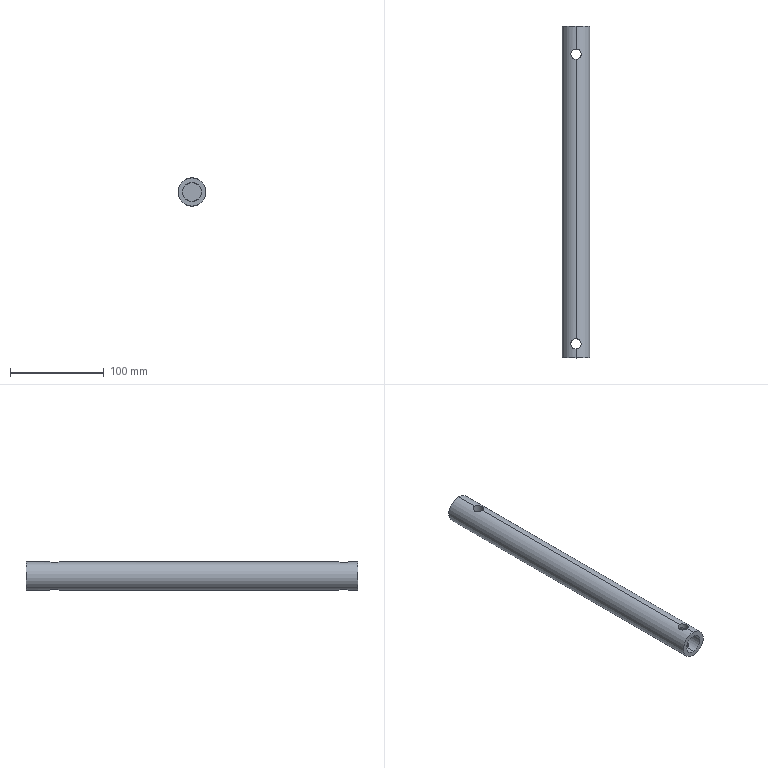Part | SolidWorks | features ICE 2, Extrusion 1, MoveFace 1 | 1 solid | 13 faces | box 30 x 354 x 30 mm | volume 230741 mm3 | cylinder 10 | plane 3 | commonest cylinder face diameters 11 x6 20 x2 30 x2
STEP:
#1=CARTESIAN_POINT('',(-5.5,324.,-13.955));
#2=VERTEX_POINT('',#1);
#3=CARTESIAN_POINT('',(0.,318.5,-15.));
#4=VERTEX_POINT('',#3);
#5=CARTESIAN_POINT('',(-5.5,324.,-13.955));
#6=CARTESIAN_POINT('',(-5.5,323.818,-13.955));
#7=CARTESIAN_POINT('',(-5.491,323.634,-13.959));
#8=CARTESIAN_POINT('',(-5.455,323.272,-13.973));
#9=CARTESIAN_POINT('',(-5.428,323.093,-13.984));
#10=CARTESIAN_POINT('',(-5.321,322.562,-14.025));
#11=CARTESIAN_POINT('',(-5.215,322.214,-14.065));
#12=CARTESIAN_POINT('',(-4.936,321.547,-14.165));
#13=CARTESIAN_POINT('',(-4.766,321.232,-14.224));
#14=CARTESIAN_POINT('',(-4.368,320.639,-14.352));
#15=CARTESIAN_POINT('',(-4.137,320.358,-14.421));
#16=CARTESIAN_POINT('',(-3.633,319.855,-14.556));
#17=CARTESIAN_POINT('',(-3.358,319.63,-14.622));
#18=CARTESIAN_POINT('',(-2.91,319.33,-14.716));
#19=CARTESIAN_POINT('',(-2.755,319.236,-14.746));
#20=CARTESIAN_POINT('',(-2.438,319.067,-14.801));
#21=CARTESIAN_POINT('',(-2.277,318.99,-14.827));
#22=CARTESIAN_POINT('',(-1.782,318.785,-14.897));
#23=CARTESIAN_POINT('',(-1.44,318.679,-14.935));
#24=CARTESIAN_POINT('',(-0.904,318.572,-14.974));
#25=CARTESIAN_POINT('',(-0.7225,318.545,-14.984));
#26=CARTESIAN_POINT('',(-0.3614,318.509,-14.997));
#27=CARTESIAN_POINT('',(-0.1808,318.5,-15.));
#28=CARTESIAN_POINT('',(0.,318.5,-15.));
#29=B_SPLINE_CURVE_WITH_KNOTS('',3,(#5,#6,#7,#8,#9,#10,#11,#12,#13,#14,#15,#16,#17,#18,#19,#20,#21,#22,#23,#24,#25,#26,#27,#28),.UNSPECIFIED.,.F.,.F.,(4,2,2,2,2,2,2,2,2,2,2,4),(0.02696,0.02751,0.02805,0.02913,0.03022,0.0313,0.03239,0.03293,0.03347,0.03456,0.0351,0.03564),.UNSPECIFIED.);
#30=EDGE_CURVE('',#2,#4,#29,.T.);
#31=ORIENTED_EDGE('',*,*,#30,.F.);
#32=CARTESIAN_POINT('',(-5.5,324.,13.955));
#33=VERTEX_POINT('',#32);
#34=CARTESIAN_POINT('',(-5.5,324.,-126.));
#35=DIRECTION('',(0.,0.,1.));
#36=VECTOR('',#35,1000.);
#37=LINE('',#34,#36);
#38=EDGE_CURVE('',#2,#33,#37,.T.);
#39=ORIENTED_EDGE('',*,*,#38,.T.);
#40=CARTESIAN_POINT('',(0.,318.5,15.));
#41=VERTEX_POINT('',#40);
#42=CARTESIAN_POINT('',(0.,318.5,15.));
#43=CARTESIAN_POINT('',(-0.182,318.5,15.));
#44=CARTESIAN_POINT('',(-0.3661,318.509,14.997));
#45=CARTESIAN_POINT('',(-0.7283,318.545,14.983));
#46=CARTESIAN_POINT('',(-0.9072,318.572,14.974));
#47=CARTESIAN_POINT('',(-1.438,318.679,14.935));
#48=CARTESIAN_POINT('',(-1.786,318.785,14.897));
#49=CARTESIAN_POINT('',(-2.454,319.065,14.802));
#50=CARTESIAN_POINT('',(-2.769,319.235,14.745));
#51=CARTESIAN_POINT('',(-3.363,319.633,14.621));
#52=CARTESIAN_POINT('',(-3.643,319.864,14.553));
#53=CARTESIAN_POINT('',(-4.146,320.369,14.418));
#54=CARTESIAN_POINT('',(-4.372,320.643,14.35));
#55=CARTESIAN_POINT('',(-4.671,321.091,14.254));
#56=CARTESIAN_POINT('',(-4.765,321.247,14.223));
#57=CARTESIAN_POINT('',(-4.934,321.563,14.166));
#58=CARTESIAN_POINT('',(-5.01,321.724,14.139));
#59=CARTESIAN_POINT('',(-5.216,322.218,14.065));
#60=CARTESIAN_POINT('',(-5.321,322.561,14.025));
#61=CARTESIAN_POINT('',(-5.428,323.096,13.983));
#62=CARTESIAN_POINT('',(-5.455,323.277,13.973));
#63=CARTESIAN_POINT('',(-5.491,323.639,13.959));
#64=CARTESIAN_POINT('',(-5.5,323.819,13.955));
#65=CARTESIAN_POINT('',(-5.5,324.,13.955));
#66=B_SPLINE_CURVE_WITH_KNOTS('',3,(#42,#43,#44,#45,#46,#47,#48,#49,#50,#51,#52,#53,#54,#55,#56,#57,#58,#59,#60,#61,#62,#63,#64,#65),.UNSPECIFIED.,.F.,.F.,(4,2,2,2,2,2,2,2,2,2,2,4),(0.02696,0.0275,0.02804,0.02912,0.03021,0.03129,0.03238,0.03292,0.03346,0.03455,0.03509,0.03563),.UNSPECIFIED.);
#67=EDGE_CURVE('',#41,#33,#66,.T.);
#68=ORIENTED_EDGE('',*,*,#67,.F.);
#69=CARTESIAN_POINT('',(5.5,324.,13.955));
#70=VERTEX_POINT('',#69);
#71=CARTESIAN_POINT('',(5.5,324.,13.955));
#72=CARTESIAN_POINT('',(5.5,323.634,13.955));
#73=CARTESIAN_POINT('',(5.464,323.275,13.97));
#74=CARTESIAN_POINT('',(5.322,322.566,14.024));
#75=CARTESIAN_POINT('',(5.214,322.214,14.065));
#76=CARTESIAN_POINT('',(4.938,321.551,14.165));
#77=CARTESIAN_POINT('',(4.769,321.236,14.223));
#78=CARTESIAN_POINT('',(4.368,320.638,14.352));
#79=CARTESIAN_POINT('',(4.14,320.361,14.42));
#80=CARTESIAN_POINT('',(3.763,319.984,14.521));
#81=CARTESIAN_POINT('',(3.631,319.865,14.555));
#82=CARTESIAN_POINT('',(3.354,319.638,14.621));
#83=CARTESIAN_POINT('',(3.209,319.529,14.654));
#84=CARTESIAN_POINT('',(2.761,319.23,14.747));
#85=CARTESIAN_POINT('',(2.447,319.061,14.803));
#86=CARTESIAN_POINT('',(1.784,318.785,14.897));
#87=CARTESIAN_POINT('',(1.432,318.677,14.936));
#88=CARTESIAN_POINT('',(0.7232,318.536,14.987));
#89=CARTESIAN_POINT('',(0.364,318.5,15.));
#90=CARTESIAN_POINT('',(0.,318.5,15.));
#91=B_SPLINE_CURVE_WITH_KNOTS('',3,(#71,#72,#73,#74,#75,#76,#77,#78,#79,#80,#81,#82,#83,#84,#85,#86,#87,#88,#89,#90),.UNSPECIFIED.,.F.,.F.,(4,2,2,2,2,2,2,2,2,4),(0.01828,0.01936,0.02045,0.02153,0.02262,0.02316,0.0237,0.02479,0.02587,0.02696),.UNSPECIFIED.);
#92=EDGE_CURVE('',#70,#41,#91,.T.);
#93=ORIENTED_EDGE('',*,*,#92,.F.);
#94=CARTESIAN_POINT('',(5.5,324.,-13.955));
#95=VERTEX_POINT('',#94);
#96=CARTESIAN_POINT('',(5.5,324.,-126.));
#97=DIRECTION('',(0.,0.,1.));
#98=VECTOR('',#97,1000.);
#99=LINE('',#96,#98);
#100=EDGE_CURVE('',#95,#70,#99,.T.);
#101=ORIENTED_EDGE('',*,*,#100,.F.);
#102=CARTESIAN_POINT('',(0.,318.5,-15.));
#103=CARTESIAN_POINT('',(0.1807,318.5,-15.));
#104=CARTESIAN_POINT('',(0.3616,318.509,-14.997));
#105=CARTESIAN_POINT('',(0.7235,318.545,-14.984));
#106=CARTESIAN_POINT('',(0.9054,318.572,-14.974));
#107=CARTESIAN_POINT('',(1.439,318.679,-14.935));
#108=CARTESIAN_POINT('',(1.783,318.785,-14.897));
#109=CARTESIAN_POINT('',(2.448,319.062,-14.803));
#110=CARTESIAN_POINT('',(2.769,319.235,-14.745));
#111=CARTESIAN_POINT('',(3.361,319.632,-14.622));
#112=CARTESIAN_POINT('',(3.637,319.858,-14.555));
#113=CARTESIAN_POINT('',(4.145,320.368,-14.418));
#114=CARTESIAN_POINT('',(4.371,320.643,-14.35));
#115=CARTESIAN_POINT('',(4.668,321.086,-14.255));
#116=CARTESIAN_POINT('',(4.76,321.239,-14.225));
#117=CARTESIAN_POINT('',(4.93,321.556,-14.167));
#118=CARTESIAN_POINT('',(5.009,321.72,-14.139));
#119=CARTESIAN_POINT('',(5.216,322.219,-14.065));
#120=CARTESIAN_POINT('',(5.321,322.562,-14.025));
#121=CARTESIAN_POINT('',(5.463,323.27,-13.97));
#122=CARTESIAN_POINT('',(5.5,323.638,-13.955));
#123=CARTESIAN_POINT('',(5.5,324.,-13.955));
#124=B_SPLINE_CURVE_WITH_KNOTS('',3,(#102,#103,#104,#105,#106,#107,#108,#109,#110,#111,#112,#113,#114,#115,#116,#117,#118,#119,#120,#121,#122,#123),.UNSPECIFIED.,.F.,.F.,(4,2,2,2,2,2,2,2,2,2,4),(0.0009354,0.001478,0.00202,0.003104,0.004189,0.005273,0.006357,0.006899,0.007442,0.008526,0.00961),.UNSPECIFIED.);
#125=EDGE_CURVE('',#4,#95,#124,.T.);
#126=ORIENTED_EDGE('',*,*,#125,.F.);
#127=EDGE_LOOP('',(#31,#39,#68,#93,#101,#126));
#128=FACE_OUTER_BOUND('',#127,.T.);
#129=CARTESIAN_POINT('',(0.,324.,-126.));
#130=DIRECTION('',(0.,0.,1.));
#131=DIRECTION('',(1.,0.,0.));
#132=AXIS2_PLACEMENT_3D('',#129,#130,#131);
#133=CYLINDRICAL_SURFACE('',#132,5.5);
#134=ADVANCED_FACE('',(#128),#133,.F.);
#135=CARTESIAN_POINT('',(-5.5,15.,-13.955));
#136=VERTEX_POINT('',#135);
#137=CARTESIAN_POINT('',(0.,9.5,-15.));
#138=VERTEX_POINT('',#137);
#139=CARTESIAN_POINT('',(-5.5,15.,-13.955));
#140=CARTESIAN_POINT('',(-5.5,14.638,-13.955));
#141=CARTESIAN_POINT('',(-5.463,14.27,-13.97));
#142=CARTESIAN_POINT('',(-5.321,13.562,-14.025));
#143=CARTESIAN_POINT('',(-5.216,13.218,-14.065));
#144=CARTESIAN_POINT('',(-4.936,12.548,-14.165));
#145=CARTESIAN_POINT('',(-4.766,12.232,-14.224));
#146=CARTESIAN_POINT('',(-4.369,11.64,-14.351));
#147=CARTESIAN_POINT('',(-4.139,11.36,-14.42));
#148=CARTESIAN_POINT('',(-3.634,10.856,-14.555));
#149=CARTESIAN_POINT('',(-3.36,10.631,-14.622));
#150=CARTESIAN_POINT('',(-2.765,10.232,-14.746));
#151=CARTESIAN_POINT('',(-2.444,10.06,-14.803));
#152=CARTESIAN_POINT('',(-1.783,9.785,-14.897));
#153=CARTESIAN_POINT('',(-1.439,9.679,-14.935));
#154=CARTESIAN_POINT('',(-0.9036,9.572,-14.974));
#155=CARTESIAN_POINT('',(-0.7221,9.545,-14.984));
#156=CARTESIAN_POINT('',(-0.3611,9.509,-14.997));
#157=CARTESIAN_POINT('',(-0.1806,9.5,-15.));
#158=CARTESIAN_POINT('',(0.,9.5,-15.));
#159=B_SPLINE_CURVE_WITH_KNOTS('',3,(#139,#140,#141,#142,#143,#144,#145,#146,#147,#148,#149,#150,#151,#152,#153,#154,#155,#156,#157,#158),.UNSPECIFIED.,.F.,.F.,(4,2,2,2,2,2,2,2,2,4),(0.008677,0.009761,0.01084,0.01193,0.01301,0.0141,0.01518,0.01626,0.01681,0.01735),.UNSPECIFIED.);
#160=EDGE_CURVE('',#136,#138,#159,.T.);
#161=ORIENTED_EDGE('',*,*,#160,.F.);
#162=CARTESIAN_POINT('',(-5.5,15.,-8.352));
#163=VERTEX_POINT('',#162);
#164=CARTESIAN_POINT('',(-5.5,15.,-126.));
#165=DIRECTION('',(0.,0.,1.));
#166=VECTOR('',#165,1000.);
#167=LINE('',#164,#166);
#168=EDGE_CURVE('',#136,#163,#167,.T.);
#169=ORIENTED_EDGE('',*,*,#168,.T.);
#170=CARTESIAN_POINT('',(0.,9.5,-10.));
#171=VERTEX_POINT('',#170);
#172=CARTESIAN_POINT('',(0.,9.5,-10.));
#173=CARTESIAN_POINT('',(-0.1836,9.5,-10.));
#174=CARTESIAN_POINT('',(-0.3694,9.509,-9.995));
#175=CARTESIAN_POINT('',(-0.7371,9.546,-9.974));
#176=CARTESIAN_POINT('',(-0.9184,9.574,-9.959));
#177=CARTESIAN_POINT('',(-1.454,9.683,-9.9));
#178=CARTESIAN_POINT('',(-1.804,9.792,-9.842));
#179=CARTESIAN_POINT('',(-2.472,10.074,-9.696));
#180=CARTESIAN_POINT('',(-2.786,10.244,-9.609));
#181=CARTESIAN_POINT('',(-3.375,10.643,-9.418));
#182=CARTESIAN_POINT('',(-3.651,10.872,-9.314));
#183=CARTESIAN_POINT('',(-4.147,11.37,-9.104));
#184=CARTESIAN_POINT('',(-4.37,11.642,-8.997));
#185=CARTESIAN_POINT('',(-4.767,12.233,-8.794));
#186=CARTESIAN_POINT('',(-4.935,12.547,-8.699));
#187=CARTESIAN_POINT('',(-5.142,13.039,-8.577));
#188=CARTESIAN_POINT('',(-5.203,13.207,-8.54));
#189=CARTESIAN_POINT('',(-5.309,13.553,-8.474));
#190=CARTESIAN_POINT('',(-5.355,13.73,-8.446));
#191=CARTESIAN_POINT('',(-5.464,14.271,-8.376));
#192=CARTESIAN_POINT('',(-5.5,14.634,-8.352));
#193=CARTESIAN_POINT('',(-5.5,15.,-8.352));
#194=B_SPLINE_CURVE_WITH_KNOTS('',3,(#172,#173,#174,#175,#176,#177,#178,#179,#180,#181,#182,#183,#184,#185,#186,#187,#188,#189,#190,#191,#192,#193),.UNSPECIFIED.,.F.,.F.,(4,2,2,2,2,2,2,2,2,2,4),(0.01757,0.01812,0.01866,0.01976,0.02086,0.02195,0.02305,0.02415,0.02469,0.02524,0.02634),.UNSPECIFIED.);
#195=EDGE_CURVE('',#171,#163,#194,.T.);
#196=ORIENTED_EDGE('',*,*,#195,.F.);
#197=CARTESIAN_POINT('',(5.5,15.,-8.352));
#198=VERTEX_POINT('',#197);
#199=CARTESIAN_POINT('',(5.5,15.,-8.352));
#200=CARTESIAN_POINT('',(5.5,14.816,-8.352));
#201=CARTESIAN_POINT('',(5.491,14.63,-8.358));
#202=CARTESIAN_POINT('',(5.454,14.263,-8.382));
#203=CARTESIAN_POINT('',(5.426,14.082,-8.4));
#204=CARTESIAN_POINT('',(5.354,13.726,-8.446));
#205=CARTESIAN_POINT('',(5.309,13.55,-8.475));
#206=CARTESIAN_POINT('',(5.201,13.203,-8.541));
#207=CARTESIAN_POINT('',(5.139,13.032,-8.579));
#208=CARTESIAN_POINT('',(4.93,12.535,-8.702));
#209=CARTESIAN_POINT('',(4.76,12.223,-8.797));
#210=CARTESIAN_POINT('',(4.364,11.633,-9.));
#211=CARTESIAN_POINT('',(4.137,11.359,-9.108));
#212=CARTESIAN_POINT('',(3.641,10.863,-9.318));
#213=CARTESIAN_POINT('',(3.367,10.636,-9.421));
#214=CARTESIAN_POINT('',(2.774,10.237,-9.613));
#215=CARTESIAN_POINT('',(2.461,10.068,-9.698));
#216=CARTESIAN_POINT('',(1.966,9.86,-9.806));
#217=CARTESIAN_POINT('',(1.796,9.798,-9.839));
#218=CARTESIAN_POINT('',(1.448,9.691,-9.896));
#219=CARTESIAN_POINT('',(1.269,9.645,-9.921));
#220=CARTESIAN_POINT('',(0.7304,9.536,-9.98));
#221=CARTESIAN_POINT('',(0.3673,9.5,-10.));
#222=CARTESIAN_POINT('',(0.,9.5,-10.));
#223=B_SPLINE_CURVE_WITH_KNOTS('',3,(#199,#200,#201,#202,#203,#204,#205,#206,#207,#208,#209,#210,#211,#212,#213,#214,#215,#216,#217,#218,#219,#220,#221,#222),.UNSPECIFIED.,.F.,.F.,(4,2,2,2,2,2,2,2,2,2,2,4),(0.008791,0.00934,0.009888,0.01044,0.01099,0.01208,0.01318,0.01428,0.01537,0.01592,0.01647,0.01757),.UNSPECIFIED.);
#224=EDGE_CURVE('',#198,#171,#223,.T.);
#225=ORIENTED_EDGE('',*,*,#224,.F.);
#226=CARTESIAN_POINT('',(5.5,15.,-13.955));
#227=VERTEX_POINT('',#226);
#228=CARTESIAN_POINT('',(5.5,15.,-126.));
#229=DIRECTION('',(0.,0.,1.));
#230=VECTOR('',#229,1000.);
#231=LINE('',#228,#230);
#232=EDGE_CURVE('',#227,#198,#231,.T.);
#233=ORIENTED_EDGE('',*,*,#232,.F.);
#234=CARTESIAN_POINT('',(0.,9.5,-15.));
#235=CARTESIAN_POINT('',(0.1806,9.5,-15.));
#236=CARTESIAN_POINT('',(0.3612,9.509,-14.997));
#237=CARTESIAN_POINT('',(0.7226,9.545,-14.984));
#238=CARTESIAN_POINT('',(0.9044,9.572,-14.974));
#239=CARTESIAN_POINT('',(1.439,9.679,-14.935));
#240=CARTESIAN_POINT('',(1.783,9.785,-14.897));
#241=CARTESIAN_POINT('',(2.448,10.062,-14.803));
#242=CARTESIAN_POINT('',(2.769,10.234,-14.745));
#243=CARTESIAN_POINT('',(3.361,10.632,-14.622));
#244=CARTESIAN_POINT('',(3.637,10.858,-14.555));
#245=CARTESIAN_POINT('',(4.145,11.367,-14.418));
#246=CARTESIAN_POINT('',(4.371,11.643,-14.35));
#247=CARTESIAN_POINT('',(4.668,12.086,-14.255));
#248=CARTESIAN_POINT('',(4.76,12.239,-14.225));
#249=CARTESIAN_POINT('',(4.93,12.555,-14.167));
#250=CARTESIAN_POINT('',(5.008,12.72,-14.139));
#251=CARTESIAN_POINT('',(5.216,13.219,-14.065));
#252=CARTESIAN_POINT('',(5.321,13.563,-14.025));
#253=CARTESIAN_POINT('',(5.463,14.27,-13.97));
#254=CARTESIAN_POINT('',(5.5,14.638,-13.955));
#255=CARTESIAN_POINT('',(5.5,15.,-13.955));
#256=B_SPLINE_CURVE_WITH_KNOTS('',3,(#234,#235,#236,#237,#238,#239,#240,#241,#242,#243,#244,#245,#246,#247,#248,#249,#250,#251,#252,#253,#254,#255),.UNSPECIFIED.,.F.,.F.,(4,2,2,2,2,2,2,2,2,2,4),(0.01735,0.01789,0.01843,0.01952,0.0206,0.02168,0.02277,0.02331,0.02385,0.02493,0.02602),.UNSPECIFIED.);
#257=EDGE_CURVE('',#138,#227,#256,.T.);
#258=ORIENTED_EDGE('',*,*,#257,.F.);
#259=EDGE_LOOP('',(#161,#169,#196,#225,#233,#258));
#260=FACE_OUTER_BOUND('',#259,.T.);
#261=CARTESIAN_POINT('',(0.,15.,-126.));
#262=DIRECTION('',(0.,0.,1.));
#263=DIRECTION('',(1.,0.,0.));
#264=AXIS2_PLACEMENT_3D('',#261,#262,#263);
#265=CYLINDRICAL_SURFACE('',#264,5.5);
#266=ADVANCED_FACE('',(#260),#265,.F.);
#267=CARTESIAN_POINT('',(-5.5,15.,8.352));
#268=VERTEX_POINT('',#267);
#269=CARTESIAN_POINT('',(0.,9.5,10.));
#270=VERTEX_POINT('',#269);
#271=CARTESIAN_POINT('',(-5.5,15.,8.352));
#272=CARTESIAN_POINT('',(-5.5,14.634,8.352));
#273=CARTESIAN_POINT('',(-5.462,14.261,8.377));
#274=CARTESIAN_POINT('',(-5.317,13.547,8.47));
#275=CARTESIAN_POINT('',(-5.209,13.199,8.538));
#276=CARTESIAN_POINT('',(-4.93,12.534,8.702));
#277=CARTESIAN_POINT('',(-4.76,12.222,8.797));
#278=CARTESIAN_POINT('',(-4.365,11.635,9.));
#279=CARTESIAN_POINT('',(-4.137,11.359,9.108));
#280=CARTESIAN_POINT('',(-3.64,10.862,9.318));
#281=CARTESIAN_POINT('',(-3.369,10.638,9.421));
#282=CARTESIAN_POINT('',(-2.775,10.238,9.612));
#283=CARTESIAN_POINT('',(-2.46,10.068,9.699));
#284=CARTESIAN_POINT('',(-1.965,9.86,9.806));
#285=CARTESIAN_POINT('',(-1.796,9.798,9.839));
#286=CARTESIAN_POINT('',(-1.45,9.691,9.896));
#287=CARTESIAN_POINT('',(-1.271,9.646,9.921));
#288=CARTESIAN_POINT('',(-0.73,9.536,9.98));
#289=CARTESIAN_POINT('',(-0.3664,9.5,10.));
#290=CARTESIAN_POINT('',(0.,9.5,10.));
#291=B_SPLINE_CURVE_WITH_KNOTS('',3,(#271,#272,#273,#274,#275,#276,#277,#278,#279,#280,#281,#282,#283,#284,#285,#286,#287,#288,#289,#290),.UNSPECIFIED.,.F.,.F.,(4,2,2,2,2,2,2,2,2,4),(0.01757,0.01866,0.01976,0.02085,0.02195,0.02304,0.02414,0.02469,0.02524,0.02633),.UNSPECIFIED.);
#292=EDGE_CURVE('',#268,#270,#291,.T.);
#293=ORIENTED_EDGE('',*,*,#292,.F.);
#294=CARTESIAN_POINT('',(-5.5,15.,13.955));
#295=VERTEX_POINT('',#294);
#296=CARTESIAN_POINT('',(-5.5,15.,-126.));
#297=DIRECTION('',(0.,0.,1.));
#298=VECTOR('',#297,1000.);
#299=LINE('',#296,#298);
#300=EDGE_CURVE('',#268,#295,#299,.T.);
#301=ORIENTED_EDGE('',*,*,#300,.T.);
#302=CARTESIAN_POINT('',(0.,9.5,15.));
#303=VERTEX_POINT('',#302);
#304=CARTESIAN_POINT('',(0.,9.5,15.));
#305=CARTESIAN_POINT('',(-0.3624,9.5,15.));
#306=CARTESIAN_POINT('',(-0.7302,9.537,14.986));
#307=CARTESIAN_POINT('',(-1.438,9.679,14.935));
#308=CARTESIAN_POINT('',(-1.783,9.784,14.898));
#309=CARTESIAN_POINT('',(-2.453,10.064,14.802));
#310=CARTESIAN_POINT('',(-2.769,10.234,14.745));
#311=CARTESIAN_POINT('',(-3.361,10.632,14.622));
#312=CARTESIAN_POINT('',(-3.641,10.862,14.554));
#313=CARTESIAN_POINT('',(-4.145,11.368,14.418));
#314=CARTESIAN_POINT('',(-4.371,11.642,14.351));
#315=CARTESIAN_POINT('',(-4.768,12.236,14.223));
#316=CARTESIAN_POINT('',(-4.941,12.557,14.164));
#317=CARTESIAN_POINT('',(-5.216,13.218,14.065));
#318=CARTESIAN_POINT('',(-5.321,13.561,14.025));
#319=CARTESIAN_POINT('',(-5.428,14.096,13.983));
#320=CARTESIAN_POINT('',(-5.455,14.278,13.973));
#321=CARTESIAN_POINT('',(-5.491,14.639,13.959));
#322=CARTESIAN_POINT('',(-5.5,14.819,13.955));
#323=CARTESIAN_POINT('',(-5.5,15.,13.955));
#324=B_SPLINE_CURVE_WITH_KNOTS('',3,(#304,#305,#306,#307,#308,#309,#310,#311,#312,#313,#314,#315,#316,#317,#318,#319,#320,#321,#322,#323),.UNSPECIFIED.,.F.,.F.,(4,2,2,2,2,2,2,2,2,4),(0.008676,0.00976,0.01084,0.01193,0.01301,0.0141,0.01518,0.01626,0.01681,0.01735),.UNSPECIFIED.);
#325=EDGE_CURVE('',#303,#295,#324,.T.);
#326=ORIENTED_EDGE('',*,*,#325,.F.);
#327=CARTESIAN_POINT('',(5.5,15.,13.955));
#328=VERTEX_POINT('',#327);
#329=CARTESIAN_POINT('',(5.5,15.,13.955));
#330=CARTESIAN_POINT('',(5.5,14.633,13.955));
#331=CARTESIAN_POINT('',(5.464,14.273,13.97));
#332=CARTESIAN_POINT('',(5.322,13.565,14.024));
#333=CARTESIAN_POINT('',(5.215,13.214,14.065));
#334=CARTESIAN_POINT('',(4.937,12.55,14.165));
#335=CARTESIAN_POINT('',(4.768,12.235,14.224));
#336=CARTESIAN_POINT('',(4.469,11.789,14.319));
#337=CARTESIAN_POINT('',(4.361,11.644,14.353));
#338=CARTESIAN_POINT('',(4.133,11.367,14.42));
#339=CARTESIAN_POINT('',(4.013,11.235,14.454));
#340=CARTESIAN_POINT('',(3.636,10.858,14.555));
#341=CARTESIAN_POINT('',(3.361,10.631,14.622));
#342=CARTESIAN_POINT('',(2.761,10.229,14.747));
#343=CARTESIAN_POINT('',(2.445,10.061,14.803));
#344=CARTESIAN_POINT('',(1.949,9.854,14.874));
#345=CARTESIAN_POINT('',(1.78,9.793,14.895));
#346=CARTESIAN_POINT('',(1.434,9.687,14.932));
#347=CARTESIAN_POINT('',(1.256,9.642,14.948));
#348=CARTESIAN_POINT('',(0.7219,9.536,14.987));
#349=CARTESIAN_POINT('',(0.3626,9.5,15.));
#350=CARTESIAN_POINT('',(0.,9.5,15.));
#351=B_SPLINE_CURVE_WITH_KNOTS('',3,(#329,#330,#331,#332,#333,#334,#335,#336,#337,#338,#339,#340,#341,#342,#343,#344,#345,#346,#347,#348,#349,#350),.UNSPECIFIED.,.F.,.F.,(4,2,2,2,2,2,2,2,2,2,4),(0.,0.001085,0.002169,0.003254,0.003796,0.004338,0.005423,0.006507,0.00705,0.007592,0.008676),.UNSPECIFIED.);
#352=EDGE_CURVE('',#328,#303,#351,.T.);
#353=ORIENTED_EDGE('',*,*,#352,.F.);
#354=CARTESIAN_POINT('',(5.5,15.,8.352));
#355=VERTEX_POINT('',#354);
#356=CARTESIAN_POINT('',(5.5,15.,-126.));
#357=DIRECTION('',(0.,0.,1.));
#358=VECTOR('',#357,1000.);
#359=LINE('',#356,#358);
#360=EDGE_CURVE('',#355,#328,#359,.T.);
#361=ORIENTED_EDGE('',*,*,#360,.F.);
#362=CARTESIAN_POINT('',(0.,9.5,10.));
#363=CARTESIAN_POINT('',(0.3658,9.5,10.));
#364=CARTESIAN_POINT('',(0.7382,9.538,9.979));
#365=CARTESIAN_POINT('',(1.453,9.683,9.9));
#366=CARTESIAN_POINT('',(1.799,9.79,9.843));
#367=CARTESIAN_POINT('',(2.47,10.072,9.696));
#368=CARTESIAN_POINT('',(2.783,10.243,9.61));
#369=CARTESIAN_POINT('',(3.371,10.64,9.42));
#370=CARTESIAN_POINT('',(3.647,10.868,9.315));
#371=CARTESIAN_POINT('',(4.144,11.367,9.105));
#372=CARTESIAN_POINT('',(4.367,11.637,8.999));
#373=CARTESIAN_POINT('',(4.663,12.078,8.847));
#374=CARTESIAN_POINT('',(4.756,12.232,8.797));
#375=CARTESIAN_POINT('',(4.925,12.545,8.704));
#376=CARTESIAN_POINT('',(5.002,12.705,8.66));
#377=CARTESIAN_POINT('',(5.208,13.197,8.538));
#378=CARTESIAN_POINT('',(5.315,13.54,8.471));
#379=CARTESIAN_POINT('',(5.462,14.259,8.377));
#380=CARTESIAN_POINT('',(5.5,14.629,8.352));
#381=CARTESIAN_POINT('',(5.5,15.,8.352));
#382=B_SPLINE_CURVE_WITH_KNOTS('',3,(#362,#363,#364,#365,#366,#367,#368,#369,#370,#371,#372,#373,#374,#375,#376,#377,#378,#379,#380,#381),.UNSPECIFIED.,.F.,.F.,(4,2,2,2,2,2,2,2,2,4),(0.02633,0.02743,0.02852,0.02961,0.03071,0.0318,0.03235,0.0329,0.03399,0.03509),.UNSPECIFIED.);
#383=EDGE_CURVE('',#270,#355,#382,.T.);
#384=ORIENTED_EDGE('',*,*,#383,.F.);
#385=EDGE_LOOP('',(#293,#301,#326,#353,#361,#384));
#386=FACE_OUTER_BOUND('',#385,.T.);
#387=CARTESIAN_POINT('',(0.,15.,-126.));
#388=DIRECTION('',(0.,0.,1.));
#389=DIRECTION('',(1.,0.,0.));
#390=AXIS2_PLACEMENT_3D('',#387,#388,#389);
#391=CYLINDRICAL_SURFACE('',#390,5.5);
#392=ADVANCED_FACE('',(#386),#391,.F.);
#393=CARTESIAN_POINT('',(0.,50.,10.));
#394=VERTEX_POINT('',#393);
#395=CARTESIAN_POINT('',(0.,50.,-10.));
#396=VERTEX_POINT('',#395);
#397=CARTESIAN_POINT('',(0.,50.,0.));
#398=DIRECTION('',(0.,-1.,0.));
#399=DIRECTION('',(0.,0.,-1.));
#400=AXIS2_PLACEMENT_3D('',#397,#398,#399);
#401=CIRCLE('',#400,10.);
#402=EDGE_CURVE('',#394,#396,#401,.T.);
#403=ORIENTED_EDGE('',*,*,#402,.F.);
#404=CARTESIAN_POINT('',(0.,20.5,10.));
#405=VERTEX_POINT('',#404);
#406=CARTESIAN_POINT('',(0.,50.,10.));
#407=DIRECTION('',(0.,-1.,0.));
#408=VECTOR('',#407,1000.);
#409=LINE('',#406,#408);
#410=EDGE_CURVE('',#394,#405,#409,.T.);
#411=ORIENTED_EDGE('',*,*,#410,.T.);
#412=CARTESIAN_POINT('',(0.,20.5,10.));
#413=CARTESIAN_POINT('',(-0.1843,20.5,10.));
#414=CARTESIAN_POINT('',(-0.3708,20.491,9.995));
#415=CARTESIAN_POINT('',(-0.7371,20.453,9.974));
#416=CARTESIAN_POINT('',(-0.918,20.426,9.959));
#417=CARTESIAN_POINT('',(-1.275,20.353,9.92));
#418=CARTESIAN_POINT('',(-1.451,20.308,9.896));
#419=CARTESIAN_POINT('',(-1.8,20.2,9.838));
#420=CARTESIAN_POINT('',(-1.972,20.137,9.805));
#421=CARTESIAN_POINT('',(-2.472,19.927,9.696));
#422=CARTESIAN_POINT('',(-2.785,19.756,9.609));
#423=CARTESIAN_POINT('',(-3.228,19.456,9.466));
#424=CARTESIAN_POINT('',(-3.372,19.349,9.416));
#425=CARTESIAN_POINT('',(-3.645,19.123,9.313));
#426=CARTESIAN_POINT('',(-3.775,19.004,9.261));
#427=CARTESIAN_POINT('',(-4.147,18.63,9.104));
#428=CARTESIAN_POINT('',(-4.371,18.357,8.997));
#429=CARTESIAN_POINT('',(-4.768,17.765,8.793));
#430=CARTESIAN_POINT('',(-4.935,17.454,8.699));
#431=CARTESIAN_POINT('',(-5.142,16.961,8.577));
#432=CARTESIAN_POINT('',(-5.203,16.792,8.54));
#433=CARTESIAN_POINT('',(-5.31,16.446,8.474));
#434=CARTESIAN_POINT('',(-5.355,16.267,8.445));
#435=CARTESIAN_POINT('',(-5.464,15.729,8.376));
#436=CARTESIAN_POINT('',(-5.5,15.367,8.352));
#437=CARTESIAN_POINT('',(-5.5,15.,8.352));
#438=B_SPLINE_CURVE_WITH_KNOTS('',3,(#412,#413,#414,#415,#416,#417,#418,#419,#420,#421,#422,#423,#424,#425,#426,#427,#428,#429,#430,#431,#432,#433,#434,#435,#436,#437),.UNSPECIFIED.,.F.,.F.,(4,2,2,2,2,2,2,2,2,2,2,2,4),(0.008787,0.009335,0.009884,0.01043,0.01098,0.01208,0.01263,0.01318,0.01427,0.01537,0.01592,0.01647,0.01757),.UNSPECIFIED.);
#439=EDGE_CURVE('',#405,#268,#438,.T.);
#440=ORIENTED_EDGE('',*,*,#439,.T.);
#441=ORIENTED_EDGE('',*,*,#292,.T.);
#442=CARTESIAN_POINT('',(0.,0.,10.));
#443=VERTEX_POINT('',#442);
#444=CARTESIAN_POINT('',(0.,50.,10.));
#445=DIRECTION('',(0.,-1.,0.));
#446=VECTOR('',#445,1000.);
#447=LINE('',#444,#446);
#448=EDGE_CURVE('',#270,#443,#447,.T.);
#449=ORIENTED_EDGE('',*,*,#448,.T.);
#450=CARTESIAN_POINT('',(0.,0.,-10.));
#451=VERTEX_POINT('',#450);
#452=CARTESIAN_POINT('',(0.,0.,0.));
#453=DIRECTION('',(0.,-1.,0.));
#454=DIRECTION('',(0.,0.,-1.));
#455=AXIS2_PLACEMENT_3D('',#452,#453,#454);
#456=CIRCLE('',#455,10.);
#457=EDGE_CURVE('',#443,#451,#456,.T.);
#458=ORIENTED_EDGE('',*,*,#457,.T.);
#459=CARTESIAN_POINT('',(0.,50.,-10.));
#460=DIRECTION('',(0.,-1.,0.));
#461=VECTOR('',#460,1000.);
#462=LINE('',#459,#461);
#463=EDGE_CURVE('',#171,#451,#462,.T.);
#464=ORIENTED_EDGE('',*,*,#463,.F.);
#465=ORIENTED_EDGE('',*,*,#195,.T.);
#466=CARTESIAN_POINT('',(0.,20.5,-10.));
#467=VERTEX_POINT('',#466);
#468=CARTESIAN_POINT('',(-5.5,15.,-8.352));
#469=CARTESIAN_POINT('',(-5.5,15.365,-8.352));
#470=CARTESIAN_POINT('',(-5.463,15.737,-8.377));
#471=CARTESIAN_POINT('',(-5.318,16.451,-8.469));
#472=CARTESIAN_POINT('',(-5.211,16.797,-8.537));
#473=CARTESIAN_POINT('',(-4.931,17.463,-8.701));
#474=CARTESIAN_POINT('',(-4.762,17.775,-8.796));
#475=CARTESIAN_POINT('',(-4.367,18.362,-8.999));
#476=CARTESIAN_POINT('',(-4.14,18.638,-9.107));
#477=CARTESIAN_POINT('',(-3.644,19.135,-9.316));
#478=CARTESIAN_POINT('',(-3.373,19.359,-9.419));
#479=CARTESIAN_POINT('',(-2.931,19.658,-9.562));
#480=CARTESIAN_POINT('',(-2.776,19.751,-9.608));
#481=CARTESIAN_POINT('',(-2.462,19.922,-9.694));
#482=CARTESIAN_POINT('',(-2.301,19.999,-9.733));
#483=CARTESIAN_POINT('',(-1.806,20.207,-9.841));
#484=CARTESIAN_POINT('',(-1.462,20.315,-9.899));
#485=CARTESIAN_POINT('',(-0.7399,20.462,-9.979));
#486=CARTESIAN_POINT('',(-0.3704,20.5,-10.));
#487=CARTESIAN_POINT('',(0.,20.5,-10.));
#488=B_SPLINE_CURVE_WITH_KNOTS('',3,(#468,#469,#470,#471,#472,#473,#474,#475,#476,#477,#478,#479,#480,#481,#482,#483,#484,#485,#486,#487),.UNSPECIFIED.,.F.,.F.,(4,2,2,2,2,2,2,2,2,4),(0.02634,0.02743,0.02853,0.02962,0.03072,0.03181,0.03236,0.0329,0.034,0.03509),.UNSPECIFIED.);
#489=EDGE_CURVE('',#163,#467,#488,.T.);
#490=ORIENTED_EDGE('',*,*,#489,.T.);
#491=CARTESIAN_POINT('',(0.,50.,-10.));
#492=DIRECTION('',(0.,-1.,0.));
#493=VECTOR('',#492,1000.);
#494=LINE('',#491,#493);
#495=EDGE_CURVE('',#396,#467,#494,.T.);
#496=ORIENTED_EDGE('',*,*,#495,.F.);
#497=EDGE_LOOP('',(#403,#411,#440,#441,#449,#458,#464,#465,#490,#496));
#498=FACE_OUTER_BOUND('',#497,.T.);
#499=CARTESIAN_POINT('',(0.,50.,0.));
#500=DIRECTION('',(0.,-1.,0.));
#501=DIRECTION('',(0.,0.,-1.));
#502=AXIS2_PLACEMENT_3D('',#499,#500,#501);
#503=CYLINDRICAL_SURFACE('',#502,10.);
#504=ADVANCED_FACE('',(#498),#503,.F.);
#505=CARTESIAN_POINT('',(0.,354.,15.));
#506=VERTEX_POINT('',#505);
#507=CARTESIAN_POINT('',(0.,354.,-15.));
#508=VERTEX_POINT('',#507);
#509=CARTESIAN_POINT('',(0.,354.,0.));
#510=DIRECTION('',(0.,1.,0.));
#511=DIRECTION('',(0.,0.,1.));
#512=AXIS2_PLACEMENT_3D('',#509,#510,#511);
#513=CIRCLE('',#512,15.);
#514=EDGE_CURVE('',#506,#508,#513,.T.);
#515=ORIENTED_EDGE('',*,*,#514,.F.);
#516=CARTESIAN_POINT('',(0.,329.5,15.));
#517=VERTEX_POINT('',#516);
#518=CARTESIAN_POINT('',(0.,656.,15.));
#519=DIRECTION('',(0.,-1.,0.));
#520=VECTOR('',#519,1000.);
#521=LINE('',#518,#520);
#522=EDGE_CURVE('',#506,#517,#521,.T.);
#523=ORIENTED_EDGE('',*,*,#522,.T.);
#524=CARTESIAN_POINT('',(0.,329.5,15.));
#525=CARTESIAN_POINT('',(0.3621,329.5,15.));
#526=CARTESIAN_POINT('',(0.7219,329.465,14.987));
#527=CARTESIAN_POINT('',(1.258,329.357,14.948));
#528=CARTESIAN_POINT('',(1.435,329.313,14.932));
#529=CARTESIAN_POINT('',(1.781,329.207,14.895));
#530=CARTESIAN_POINT('',(1.95,329.146,14.874));
#531=CARTESIAN_POINT('',(2.281,329.008,14.826));
#532=CARTESIAN_POINT('',(2.443,328.931,14.801));
#533=CARTESIAN_POINT('',(2.76,328.76,14.745));
#534=CARTESIAN_POINT('',(2.916,328.667,14.715));
#535=CARTESIAN_POINT('',(3.363,328.367,14.621));
#536=CARTESIAN_POINT('',(3.637,328.141,14.555));
#537=CARTESIAN_POINT('',(4.142,327.636,14.419));
#538=CARTESIAN_POINT('',(4.372,327.356,14.35));
#539=CARTESIAN_POINT('',(4.768,326.764,14.223));
#540=CARTESIAN_POINT('',(4.937,326.45,14.165));
#541=CARTESIAN_POINT('',(5.146,325.949,14.09));
#542=CARTESIAN_POINT('',(5.208,325.778,14.067));
#543=CARTESIAN_POINT('',(5.313,325.433,14.028));
#544=CARTESIAN_POINT('',(5.401,325.084,13.994));
#545=CARTESIAN_POINT('',(5.455,324.727,13.973));
#546=CARTESIAN_POINT('',(5.491,324.366,13.959));
#547=CARTESIAN_POINT('',(5.5,324.183,13.955));
#548=CARTESIAN_POINT('',(5.5,324.,13.955));
#549=B_SPLINE_CURVE_WITH_KNOTS('',3,(#524,#525,#526,#527,#528,#529,#530,#531,#532,#533,#534,#535,#536,#537,#538,#539,#540,#541,#542,#543,#544,#545,#546,#547,#548),.UNSPECIFIED.,.F.,.F.,(4,2,2,2,2,2,2,2,2,2,1,2,4),(0.009602,0.01069,0.01123,0.01177,0.01231,0.01286,0.01394,0.01503,0.01611,0.01665,0.01719,0.01774,0.01828),.UNSPECIFIED.);
#550=EDGE_CURVE('',#517,#70,#549,.T.);
#551=ORIENTED_EDGE('',*,*,#550,.T.);
#552=ORIENTED_EDGE('',*,*,#92,.T.);
#553=CARTESIAN_POINT('',(0.,20.5,15.));
#554=VERTEX_POINT('',#553);
#555=CARTESIAN_POINT('',(0.,656.,15.));
#556=DIRECTION('',(0.,-1.,0.));
#557=VECTOR('',#556,1000.);
#558=LINE('',#555,#557);
#559=EDGE_CURVE('',#41,#554,#558,.T.);
#560=ORIENTED_EDGE('',*,*,#559,.T.);
#561=CARTESIAN_POINT('',(0.,20.5,15.));
#562=CARTESIAN_POINT('',(0.3625,20.5,15.));
#563=CARTESIAN_POINT('',(0.7223,20.465,14.987));
#564=CARTESIAN_POINT('',(1.258,20.357,14.948));
#565=CARTESIAN_POINT('',(1.435,20.312,14.932));
#566=CARTESIAN_POINT('',(1.781,20.207,14.895));
#567=CARTESIAN_POINT('',(1.951,20.146,14.874));
#568=CARTESIAN_POINT('',(2.282,20.007,14.826));
#569=CARTESIAN_POINT('',(2.444,19.93,14.8));
#570=CARTESIAN_POINT('',(2.761,19.76,14.745));
#571=CARTESIAN_POINT('',(2.917,19.666,14.714));
#572=CARTESIAN_POINT('',(3.364,19.366,14.621));
#573=CARTESIAN_POINT('',(3.639,19.14,14.554));
#574=CARTESIAN_POINT('',(4.143,18.635,14.419));
#575=CARTESIAN_POINT('',(4.373,18.355,14.35));
#576=CARTESIAN_POINT('',(4.769,17.762,14.223));
#577=CARTESIAN_POINT('',(4.938,17.448,14.165));
#578=CARTESIAN_POINT('',(5.147,16.948,14.09));
#579=CARTESIAN_POINT('',(5.209,16.776,14.067));
#580=CARTESIAN_POINT('',(5.314,16.43,14.027));
#581=CARTESIAN_POINT('',(5.358,16.256,14.011));
#582=CARTESIAN_POINT('',(5.464,15.727,13.97));
#583=CARTESIAN_POINT('',(5.5,15.367,13.955));
#584=CARTESIAN_POINT('',(5.5,15.,13.955));
#585=B_SPLINE_CURVE_WITH_KNOTS('',3,(#561,#562,#563,#564,#565,#566,#567,#568,#569,#570,#571,#572,#573,#574,#575,#576,#577,#578,#579,#580,#581,#582,#583,#584),.UNSPECIFIED.,.F.,.F.,(4,2,2,2,2,2,2,2,2,2,2,4),(0.02602,0.0271,0.02764,0.02819,0.02873,0.02927,0.03035,0.03144,0.03252,0.03306,0.03361,0.03469),.UNSPECIFIED.);
#586=EDGE_CURVE('',#554,#328,#585,.T.);
#587=ORIENTED_EDGE('',*,*,#586,.T.);
#588=ORIENTED_EDGE('',*,*,#352,.T.);
#589=CARTESIAN_POINT('',(0.,0.,15.));
#590=VERTEX_POINT('',#589);
#591=CARTESIAN_POINT('',(0.,656.,15.));
#592=DIRECTION('',(0.,-1.,0.));
#593=VECTOR('',#592,1000.);
#594=LINE('',#591,#593);
#595=EDGE_CURVE('',#303,#590,#594,.T.);
#596=ORIENTED_EDGE('',*,*,#595,.T.);
#597=CARTESIAN_POINT('',(0.,0.,-15.));
#598=VERTEX_POINT('',#597);
#599=CARTESIAN_POINT('',(0.,0.,0.));
#600=DIRECTION('',(0.,1.,0.));
#601=DIRECTION('',(0.,0.,1.));
#602=AXIS2_PLACEMENT_3D('',#599,#600,#601);
#603=CIRCLE('',#602,15.);
#604=EDGE_CURVE('',#590,#598,#603,.T.);
#605=ORIENTED_EDGE('',*,*,#604,.T.);
#606=CARTESIAN_POINT('',(0.,656.,-15.));
#607=DIRECTION('',(0.,-1.,0.));
#608=VECTOR('',#607,1000.);
#609=LINE('',#606,#608);
#610=EDGE_CURVE('',#138,#598,#609,.T.);
#611=ORIENTED_EDGE('',*,*,#610,.F.);
#612=ORIENTED_EDGE('',*,*,#257,.T.);
#613=CARTESIAN_POINT('',(0.,20.5,-15.));
#614=VERTEX_POINT('',#613);
#615=CARTESIAN_POINT('',(5.5,15.,-13.955));
#616=CARTESIAN_POINT('',(5.5,15.363,-13.955));
#617=CARTESIAN_POINT('',(5.465,15.722,-13.969));
#618=CARTESIAN_POINT('',(5.357,16.257,-14.011));
#619=CARTESIAN_POINT('',(5.313,16.435,-14.028));
#620=CARTESIAN_POINT('',(5.207,16.781,-14.067));
#621=CARTESIAN_POINT('',(5.146,16.95,-14.09));
#622=CARTESIAN_POINT('',(5.008,17.281,-14.14));
#623=CARTESIAN_POINT('',(4.931,17.443,-14.167));
#624=CARTESIAN_POINT('',(4.761,17.76,-14.225));
#625=CARTESIAN_POINT('',(4.667,17.915,-14.256));
#626=CARTESIAN_POINT('',(4.367,18.362,-14.352));
#627=CARTESIAN_POINT('',(4.141,18.637,-14.419));
#628=CARTESIAN_POINT('',(3.637,19.141,-14.555));
#629=CARTESIAN_POINT('',(3.356,19.372,-14.623));
#630=CARTESIAN_POINT('',(2.763,19.769,-14.746));
#631=CARTESIAN_POINT('',(2.449,19.938,-14.803));
#632=CARTESIAN_POINT('',(1.948,20.147,-14.874));
#633=CARTESIAN_POINT('',(1.776,20.208,-14.895));
#634=CARTESIAN_POINT('',(1.431,20.314,-14.933));
#635=CARTESIAN_POINT('',(1.256,20.358,-14.948));
#636=CARTESIAN_POINT('',(0.7268,20.464,-14.987));
#637=CARTESIAN_POINT('',(0.3669,20.5,-15.));
#638=CARTESIAN_POINT('',(0.,20.5,-15.));
#639=B_SPLINE_CURVE_WITH_KNOTS('',3,(#615,#616,#617,#618,#619,#620,#621,#622,#623,#624,#625,#626,#627,#628,#629,#630,#631,#632,#633,#634,#635,#636,#637,#638),.UNSPECIFIED.,.F.,.F.,(4,2,2,2,2,2,2,2,2,2,2,4),(0.02602,0.0271,0.02764,0.02819,0.02873,0.02927,0.03036,0.03144,0.03252,0.03307,0.03361,0.03469),.UNSPECIFIED.);
#640=EDGE_CURVE('',#227,#614,#639,.T.);
#641=ORIENTED_EDGE('',*,*,#640,.T.);
#642=CARTESIAN_POINT('',(0.,656.,-15.));
#643=DIRECTION('',(0.,-1.,0.));
#644=VECTOR('',#643,1000.);
#645=LINE('',#642,#644);
#646=EDGE_CURVE('',#4,#614,#645,.T.);
#647=ORIENTED_EDGE('',*,*,#646,.F.);
#648=ORIENTED_EDGE('',*,*,#125,.T.);
#649=CARTESIAN_POINT('',(0.,329.5,-15.));
#650=VERTEX_POINT('',#649);
#651=CARTESIAN_POINT('',(5.5,324.,-13.955));
#652=CARTESIAN_POINT('',(5.5,324.362,-13.955));
#653=CARTESIAN_POINT('',(5.465,324.722,-13.969));
#654=CARTESIAN_POINT('',(5.357,325.257,-14.011));
#655=CARTESIAN_POINT('',(5.313,325.435,-14.028));
#656=CARTESIAN_POINT('',(5.207,325.78,-14.067));
#657=CARTESIAN_POINT('',(5.146,325.949,-14.09));
#658=CARTESIAN_POINT('',(5.008,326.28,-14.139));
#659=CARTESIAN_POINT('',(4.931,326.442,-14.167));
#660=CARTESIAN_POINT('',(4.761,326.759,-14.225));
#661=CARTESIAN_POINT('',(4.668,326.915,-14.256));
#662=CARTESIAN_POINT('',(4.368,327.361,-14.351));
#663=CARTESIAN_POINT('',(4.142,327.636,-14.419));
#664=CARTESIAN_POINT('',(3.638,328.14,-14.554));
#665=CARTESIAN_POINT('',(3.358,328.371,-14.622));
#666=CARTESIAN_POINT('',(2.765,328.768,-14.746));
#667=CARTESIAN_POINT('',(2.451,328.937,-14.802));
#668=CARTESIAN_POINT('',(1.95,329.146,-14.874));
#669=CARTESIAN_POINT('',(1.778,329.208,-14.895));
#670=CARTESIAN_POINT('',(1.433,329.313,-14.932));
#671=CARTESIAN_POINT('',(1.084,329.401,-14.964));
#672=CARTESIAN_POINT('',(0.7269,329.455,-14.983));
#673=CARTESIAN_POINT('',(0.3661,329.491,-14.997));
#674=CARTESIAN_POINT('',(0.1827,329.5,-15.));
#675=CARTESIAN_POINT('',(0.,329.5,-15.));
#676=B_SPLINE_CURVE_WITH_KNOTS('',3,(#651,#652,#653,#654,#655,#656,#657,#658,#659,#660,#661,#662,#663,#664,#665,#666,#667,#668,#669,#670,#671,#672,#673,#674,#675),.UNSPECIFIED.,.F.,.F.,(4,2,2,2,2,2,2,2,2,2,1,2,4),(0.00961,0.01069,0.01124,0.01178,0.01232,0.01286,0.01395,0.01503,0.01612,0.01666,0.0172,0.01774,0.01829),.UNSPECIFIED.);
#677=EDGE_CURVE('',#95,#650,#676,.T.);
#678=ORIENTED_EDGE('',*,*,#677,.T.);
#679=CARTESIAN_POINT('',(0.,656.,-15.));
#680=DIRECTION('',(0.,-1.,0.));
#681=VECTOR('',#680,1000.);
#682=LINE('',#679,#681);
#683=EDGE_CURVE('',#508,#650,#682,.T.);
#684=ORIENTED_EDGE('',*,*,#683,.F.);
#685=EDGE_LOOP('',(#515,#523,#551,#552,#560,#587,#588,#596,#605,#611,#612,#641,#647,#648,#678,#684));
#686=FACE_OUTER_BOUND('',#685,.T.);
#687=CARTESIAN_POINT('',(0.,656.,0.));
#688=DIRECTION('',(0.,-1.,0.));
#689=DIRECTION('',(0.,0.,-1.));
#690=AXIS2_PLACEMENT_3D('',#687,#688,#689);
#691=CYLINDRICAL_SURFACE('',#690,15.);
#692=ADVANCED_FACE('',(#686),#691,.T.);
#693=ORIENTED_EDGE('',*,*,#522,.F.);
#694=CARTESIAN_POINT('',(0.,354.,0.));
#695=DIRECTION('',(0.,1.,0.));
#696=DIRECTION('',(0.,0.,1.));
#697=AXIS2_PLACEMENT_3D('',#694,#695,#696);
#698=CIRCLE('',#697,15.);
#699=EDGE_CURVE('',#508,#506,#698,.T.);
#700=ORIENTED_EDGE('',*,*,#699,.F.);
#701=ORIENTED_EDGE('',*,*,#683,.T.);
#702=CARTESIAN_POINT('',(0.,329.5,-15.));
#703=CARTESIAN_POINT('',(-0.3655,329.5,-15.));
#704=CARTESIAN_POINT('',(-0.7254,329.464,-14.987));
#705=CARTESIAN_POINT('',(-1.434,329.322,-14.935));
#706=CARTESIAN_POINT('',(-1.786,329.214,-14.897));
#707=CARTESIAN_POINT('',(-2.45,328.937,-14.802));
#708=CARTESIAN_POINT('',(-2.765,328.768,-14.746));
#709=CARTESIAN_POINT('',(-3.363,328.367,-14.621));
#710=CARTESIAN_POINT('',(-3.64,328.138,-14.554));
#711=CARTESIAN_POINT('',(-4.017,327.761,-14.453));
#712=CARTESIAN_POINT('',(-4.137,327.629,-14.419));
#713=CARTESIAN_POINT('',(-4.364,327.353,-14.352));
#714=CARTESIAN_POINT('',(-4.472,327.207,-14.318));
#715=CARTESIAN_POINT('',(-4.771,326.76,-14.223));
#716=CARTESIAN_POINT('',(-4.939,326.445,-14.164));
#717=CARTESIAN_POINT('',(-5.215,325.784,-14.065));
#718=CARTESIAN_POINT('',(-5.323,325.432,-14.024));
#719=CARTESIAN_POINT('',(-5.464,324.723,-13.97));
#720=CARTESIAN_POINT('',(-5.5,324.364,-13.955));
#721=CARTESIAN_POINT('',(-5.5,324.,-13.955));
#722=B_SPLINE_CURVE_WITH_KNOTS('',3,(#702,#703,#704,#705,#706,#707,#708,#709,#710,#711,#712,#713,#714,#715,#716,#717,#718,#719,#720,#721),.UNSPECIFIED.,.F.,.F.,(4,2,2,2,2,2,2,2,2,4),(0.01829,0.01937,0.02046,0.02154,0.02263,0.02317,0.02371,0.02479,0.02588,0.02696),.UNSPECIFIED.);
#723=EDGE_CURVE('',#650,#2,#722,.T.);
#724=ORIENTED_EDGE('',*,*,#723,.T.);
#725=ORIENTED_EDGE('',*,*,#30,.T.);
#726=ORIENTED_EDGE('',*,*,#646,.T.);
#727=CARTESIAN_POINT('',(0.,20.5,-15.));
#728=CARTESIAN_POINT('',(-0.367,20.5,-15.));
#729=CARTESIAN_POINT('',(-0.7272,20.464,-14.987));
#730=CARTESIAN_POINT('',(-1.435,20.322,-14.935));
#731=CARTESIAN_POINT('',(-1.786,20.214,-14.897));
#732=CARTESIAN_POINT('',(-2.451,19.937,-14.802));
#733=CARTESIAN_POINT('',(-2.766,19.767,-14.746));
#734=CARTESIAN_POINT('',(-3.213,19.468,-14.653));
#735=CARTESIAN_POINT('',(-3.358,19.36,-14.62));
#736=CARTESIAN_POINT('',(-3.635,19.132,-14.554));
#737=CARTESIAN_POINT('',(-3.767,19.012,-14.52));
#738=CARTESIAN_POINT('',(-4.143,18.634,-14.419));
#739=CARTESIAN_POINT('',(-4.37,18.359,-14.351));
#740=CARTESIAN_POINT('',(-4.771,17.759,-14.222));
#741=CARTESIAN_POINT('',(-4.94,17.444,-14.164));
#742=CARTESIAN_POINT('',(-5.146,16.949,-14.09));
#743=CARTESIAN_POINT('',(-5.207,16.78,-14.067));
#744=CARTESIAN_POINT('',(-5.313,16.433,-14.028));
#745=CARTESIAN_POINT('',(-5.358,16.256,-14.011));
#746=CARTESIAN_POINT('',(-5.465,15.722,-13.969));
#747=CARTESIAN_POINT('',(-5.5,15.363,-13.955));
#748=CARTESIAN_POINT('',(-5.5,15.,-13.955));
#749=B_SPLINE_CURVE_WITH_KNOTS('',3,(#727,#728,#729,#730,#731,#732,#733,#734,#735,#736,#737,#738,#739,#740,#741,#742,#743,#744,#745,#746,#747,#748),.UNSPECIFIED.,.F.,.F.,(4,2,2,2,2,2,2,2,2,2,4),(0.,0.001085,0.002169,0.003254,0.003796,0.004339,0.005423,0.006508,0.00705,0.007592,0.008677),.UNSPECIFIED.);
#750=EDGE_CURVE('',#614,#136,#749,.T.);
#751=ORIENTED_EDGE('',*,*,#750,.T.);
#752=ORIENTED_EDGE('',*,*,#160,.T.);
#753=ORIENTED_EDGE('',*,*,#610,.T.);
#754=CARTESIAN_POINT('',(0.,0.,0.));
#755=DIRECTION('',(0.,1.,0.));
#756=DIRECTION('',(0.,0.,1.));
#757=AXIS2_PLACEMENT_3D('',#754,#755,#756);
#758=CIRCLE('',#757,15.);
#759=EDGE_CURVE('',#598,#590,#758,.T.);
#760=ORIENTED_EDGE('',*,*,#759,.T.);
#761=ORIENTED_EDGE('',*,*,#595,.F.);
#762=ORIENTED_EDGE('',*,*,#325,.T.);
#763=CARTESIAN_POINT('',(-5.5,15.,13.955));
#764=CARTESIAN_POINT('',(-5.5,15.181,13.955));
#765=CARTESIAN_POINT('',(-5.491,15.361,13.959));
#766=CARTESIAN_POINT('',(-5.455,15.722,13.973));
#767=CARTESIAN_POINT('',(-5.428,15.904,13.983));
#768=CARTESIAN_POINT('',(-5.321,16.439,14.025));
#769=CARTESIAN_POINT('',(-5.215,16.783,14.065));
#770=CARTESIAN_POINT('',(-4.939,17.447,14.164));
#771=CARTESIAN_POINT('',(-4.766,17.767,14.224));
#772=CARTESIAN_POINT('',(-4.369,18.36,14.351));
#773=CARTESIAN_POINT('',(-4.143,18.635,14.419));
#774=CARTESIAN_POINT('',(-3.635,19.143,14.555));
#775=CARTESIAN_POINT('',(-3.359,19.37,14.622));
#776=CARTESIAN_POINT('',(-2.915,19.667,14.715));
#777=CARTESIAN_POINT('',(-2.762,19.759,14.744));
#778=CARTESIAN_POINT('',(-2.446,19.93,14.8));
#779=CARTESIAN_POINT('',(-2.281,20.008,14.826));
#780=CARTESIAN_POINT('',(-1.781,20.216,14.898));
#781=CARTESIAN_POINT('',(-1.438,20.321,14.935));
#782=CARTESIAN_POINT('',(-0.7304,20.463,14.986));
#783=CARTESIAN_POINT('',(-0.3623,20.5,15.));
#784=CARTESIAN_POINT('',(0.,20.5,15.));
#785=B_SPLINE_CURVE_WITH_KNOTS('',3,(#763,#764,#765,#766,#767,#768,#769,#770,#771,#772,#773,#774,#775,#776,#777,#778,#779,#780,#781,#782,#783,#784),.UNSPECIFIED.,.F.,.F.,(4,2,2,2,2,2,2,2,2,2,4),(0.01735,0.01789,0.01843,0.01951,0.0206,0.02168,0.02277,0.02331,0.02385,0.02493,0.02602),.UNSPECIFIED.);
#786=EDGE_CURVE('',#295,#554,#785,.T.);
#787=ORIENTED_EDGE('',*,*,#786,.T.);
#788=ORIENTED_EDGE('',*,*,#559,.F.);
#789=ORIENTED_EDGE('',*,*,#67,.T.);
#790=CARTESIAN_POINT('',(-5.5,324.,13.955));
#791=CARTESIAN_POINT('',(-5.5,324.181,13.955));
#792=CARTESIAN_POINT('',(-5.491,324.362,13.959));
#793=CARTESIAN_POINT('',(-5.455,324.723,13.973));
#794=CARTESIAN_POINT('',(-5.428,324.905,13.983));
#795=CARTESIAN_POINT('',(-5.321,325.439,14.025));
#796=CARTESIAN_POINT('',(-5.215,325.783,14.065));
#797=CARTESIAN_POINT('',(-4.939,326.447,14.164));
#798=CARTESIAN_POINT('',(-4.766,326.768,14.224));
#799=CARTESIAN_POINT('',(-4.369,327.36,14.351));
#800=CARTESIAN_POINT('',(-4.143,327.635,14.419));
#801=CARTESIAN_POINT('',(-3.634,328.144,14.556));
#802=CARTESIAN_POINT('',(-3.359,328.37,14.622));
#803=CARTESIAN_POINT('',(-2.915,328.667,14.715));
#804=CARTESIAN_POINT('',(-2.762,328.76,14.744));
#805=CARTESIAN_POINT('',(-2.445,328.93,14.8));
#806=CARTESIAN_POINT('',(-2.281,329.008,14.827));
#807=CARTESIAN_POINT('',(-1.781,329.216,14.898));
#808=CARTESIAN_POINT('',(-1.438,329.321,14.935));
#809=CARTESIAN_POINT('',(-0.7301,329.463,14.986));
#810=CARTESIAN_POINT('',(-0.3621,329.5,15.));
#811=CARTESIAN_POINT('',(0.,329.5,15.));
#812=B_SPLINE_CURVE_WITH_KNOTS('',3,(#790,#791,#792,#793,#794,#795,#796,#797,#798,#799,#800,#801,#802,#803,#804,#805,#806,#807,#808,#809,#810,#811),.UNSPECIFIED.,.F.,.F.,(4,2,2,2,2,2,2,2,2,2,4),(0.0009274,0.00147,0.002012,0.003096,0.00418,0.005265,0.006349,0.006891,0.007434,0.008518,0.009602),.UNSPECIFIED.);
#813=EDGE_CURVE('',#33,#517,#812,.T.);
#814=ORIENTED_EDGE('',*,*,#813,.T.);
#815=EDGE_LOOP('',(#693,#700,#701,#724,#725,#726,#751,#752,#753,#760,#761,#762,#787,#788,#789,#814));
#816=FACE_OUTER_BOUND('',#815,.T.);
#817=CARTESIAN_POINT('',(0.,656.,0.));
#818=DIRECTION('',(0.,-1.,0.));
#819=DIRECTION('',(0.,0.,-1.));
#820=AXIS2_PLACEMENT_3D('',#817,#818,#819);
#821=CYLINDRICAL_SURFACE('',#820,15.);
#822=ADVANCED_FACE('',(#816),#821,.T.);
#823=ORIENTED_EDGE('',*,*,#699,.T.);
#824=ORIENTED_EDGE('',*,*,#514,.T.);
#825=EDGE_LOOP('',(#823,#824));
#826=FACE_OUTER_BOUND('',#825,.T.);
#827=CARTESIAN_POINT('',(0.,354.,0.));
#828=DIRECTION('',(0.,1.,0.));
#829=DIRECTION('',(0.,0.,1.));
#830=AXIS2_PLACEMENT_3D('',#827,#828,#829);
#831=PLANE('',#830);
#832=ADVANCED_FACE('',(#826),#831,.T.);
#833=CARTESIAN_POINT('',(0.,0.,0.));
#834=DIRECTION('',(0.,-1.,0.));
#835=DIRECTION('',(0.,0.,-1.));
#836=AXIS2_PLACEMENT_3D('',#833,#834,#835);
#837=CIRCLE('',#836,10.);
#838=EDGE_CURVE('',#451,#443,#837,.T.);
#839=ORIENTED_EDGE('',*,*,#838,.F.);
#840=ORIENTED_EDGE('',*,*,#457,.F.);
#841=EDGE_LOOP('',(#839,#840));
#842=FACE_BOUND('',#841,.T.);
#843=ORIENTED_EDGE('',*,*,#759,.F.);
#844=ORIENTED_EDGE('',*,*,#604,.F.);
#845=EDGE_LOOP('',(#843,#844));
#846=FACE_OUTER_BOUND('',#845,.T.);
#847=CARTESIAN_POINT('',(0.,0.,0.));
#848=DIRECTION('',(0.,1.,0.));
#849=DIRECTION('',(0.,0.,1.));
#850=AXIS2_PLACEMENT_3D('',#847,#848,#849);
#851=PLANE('',#850);
#852=ADVANCED_FACE('',(#842,#846),#851,.F.);
#853=ORIENTED_EDGE('',*,*,#410,.F.);
#854=CARTESIAN_POINT('',(0.,50.,0.));
#855=DIRECTION('',(0.,-1.,0.));
#856=DIRECTION('',(0.,0.,-1.));
#857=AXIS2_PLACEMENT_3D('',#854,#855,#856);
#858=CIRCLE('',#857,10.);
#859=EDGE_CURVE('',#396,#394,#858,.T.);
#860=ORIENTED_EDGE('',*,*,#859,.F.);
#861=ORIENTED_EDGE('',*,*,#495,.T.);
#862=CARTESIAN_POINT('',(0.,20.5,-10.));
#863=CARTESIAN_POINT('',(0.372,20.5,-10.));
#864=CARTESIAN_POINT('',(0.7365,20.463,-9.979));
#865=CARTESIAN_POINT('',(1.451,20.318,-9.901));
#866=CARTESIAN_POINT('',(1.805,20.208,-9.842));
#867=CARTESIAN_POINT('',(2.469,19.928,-9.696));
#868=CARTESIAN_POINT('',(2.783,19.757,-9.61));
#869=CARTESIAN_POINT('',(3.376,19.357,-9.418));
#870=CARTESIAN_POINT('',(3.649,19.13,-9.314));
#871=CARTESIAN_POINT('',(4.022,18.756,-9.157));
#872=CARTESIAN_POINT('',(4.14,18.626,-9.104));
#873=CARTESIAN_POINT('',(4.364,18.352,-8.998));
#874=CARTESIAN_POINT('',(4.471,18.209,-8.946));
#875=CARTESIAN_POINT('',(4.767,17.767,-8.794));
#876=CARTESIAN_POINT('',(4.934,17.456,-8.699));
#877=CARTESIAN_POINT('',(5.21,16.797,-8.537));
#878=CARTESIAN_POINT('',(5.32,16.444,-8.468));
#879=CARTESIAN_POINT('',(5.463,15.731,-8.376));
#880=CARTESIAN_POINT('',(5.5,15.368,-8.352));
#881=CARTESIAN_POINT('',(5.5,15.,-8.352));
#882=B_SPLINE_CURVE_WITH_KNOTS('',3,(#862,#863,#864,#865,#866,#867,#868,#869,#870,#871,#872,#873,#874,#875,#876,#877,#878,#879,#880,#881),.UNSPECIFIED.,.F.,.F.,(4,2,2,2,2,2,2,2,2,4),(0.,0.001099,0.002198,0.003297,0.004396,0.004945,0.005494,0.006593,0.007692,0.008791),.UNSPECIFIED.);
#883=EDGE_CURVE('',#467,#198,#882,.T.);
#884=ORIENTED_EDGE('',*,*,#883,.T.);
#885=ORIENTED_EDGE('',*,*,#224,.T.);
#886=ORIENTED_EDGE('',*,*,#463,.T.);
#887=ORIENTED_EDGE('',*,*,#838,.T.);
#888=ORIENTED_EDGE('',*,*,#448,.F.);
#889=ORIENTED_EDGE('',*,*,#383,.T.);
#890=CARTESIAN_POINT('',(5.5,15.,8.352));
#891=CARTESIAN_POINT('',(5.5,15.372,8.352));
#892=CARTESIAN_POINT('',(5.463,15.736,8.377));
#893=CARTESIAN_POINT('',(5.318,16.449,8.469));
#894=CARTESIAN_POINT('',(5.209,16.801,8.538));
#895=CARTESIAN_POINT('',(4.931,17.462,8.701));
#896=CARTESIAN_POINT('',(4.762,17.775,8.796));
#897=CARTESIAN_POINT('',(4.364,18.366,9.));
#898=CARTESIAN_POINT('',(4.139,18.639,9.107));
#899=CARTESIAN_POINT('',(3.767,19.012,9.264));
#900=CARTESIAN_POINT('',(3.636,19.13,9.317));
#901=CARTESIAN_POINT('',(3.363,19.356,9.419));
#902=CARTESIAN_POINT('',(3.219,19.463,9.469));
#903=CARTESIAN_POINT('',(2.776,19.761,9.612));
#904=CARTESIAN_POINT('',(2.463,19.931,9.698));
#905=CARTESIAN_POINT('',(1.802,20.209,9.842));
#906=CARTESIAN_POINT('',(1.447,20.319,9.901));
#907=CARTESIAN_POINT('',(0.732,20.463,9.98));
#908=CARTESIAN_POINT('',(0.3689,20.5,10.));
#909=CARTESIAN_POINT('',(0.,20.5,10.));
#910=B_SPLINE_CURVE_WITH_KNOTS('',3,(#890,#891,#892,#893,#894,#895,#896,#897,#898,#899,#900,#901,#902,#903,#904,#905,#906,#907,#908,#909),.UNSPECIFIED.,.F.,.F.,(4,2,2,2,2,2,2,2,2,4),(0.,0.001098,0.002197,0.003295,0.004393,0.004942,0.005492,0.00659,0.007688,0.008787),.UNSPECIFIED.);
#911=EDGE_CURVE('',#355,#405,#910,.T.);
#912=ORIENTED_EDGE('',*,*,#911,.T.);
#913=EDGE_LOOP('',(#853,#860,#861,#884,#885,#886,#887,#888,#889,#912));
#914=FACE_OUTER_BOUND('',#913,.T.);
#915=CARTESIAN_POINT('',(0.,50.,0.));
#916=DIRECTION('',(0.,-1.,0.));
#917=DIRECTION('',(0.,0.,-1.));
#918=AXIS2_PLACEMENT_3D('',#915,#916,#917);
#919=CYLINDRICAL_SURFACE('',#918,10.);
#920=ADVANCED_FACE('',(#914),#919,.F.);
#921=ORIENTED_EDGE('',*,*,#859,.T.);
#922=ORIENTED_EDGE('',*,*,#402,.T.);
#923=EDGE_LOOP('',(#921,#922));
#924=FACE_OUTER_BOUND('',#923,.T.);
#925=CARTESIAN_POINT('',(0.,50.,0.));
#926=DIRECTION('',(0.,-1.,0.));
#927=DIRECTION('',(0.,0.,-1.));
#928=AXIS2_PLACEMENT_3D('',#925,#926,#927);
#929=PLANE('',#928);
#930=ADVANCED_FACE('',(#924),#929,.T.);
#931=ORIENTED_EDGE('',*,*,#300,.F.);
#932=ORIENTED_EDGE('',*,*,#439,.F.);
#933=ORIENTED_EDGE('',*,*,#911,.F.);
#934=ORIENTED_EDGE('',*,*,#360,.T.);
#935=ORIENTED_EDGE('',*,*,#586,.F.);
#936=ORIENTED_EDGE('',*,*,#786,.F.);
#937=EDGE_LOOP('',(#931,#932,#933,#934,#935,#936));
#938=FACE_OUTER_BOUND('',#937,.T.);
#939=CARTESIAN_POINT('',(0.,15.,-126.));
#940=DIRECTION('',(0.,0.,1.));
#941=DIRECTION('',(1.,0.,0.));
#942=AXIS2_PLACEMENT_3D('',#939,#940,#941);
#943=CYLINDRICAL_SURFACE('',#942,5.5);
#944=ADVANCED_FACE('',(#938),#943,.F.);
#945=ORIENTED_EDGE('',*,*,#168,.F.);
#946=ORIENTED_EDGE('',*,*,#750,.F.);
#947=ORIENTED_EDGE('',*,*,#640,.F.);
#948=ORIENTED_EDGE('',*,*,#232,.T.);
#949=ORIENTED_EDGE('',*,*,#883,.F.);
#950=ORIENTED_EDGE('',*,*,#489,.F.);
#951=EDGE_LOOP('',(#945,#946,#947,#948,#949,#950));
#952=FACE_OUTER_BOUND('',#951,.T.);
#953=CARTESIAN_POINT('',(0.,15.,-126.));
#954=DIRECTION('',(0.,0.,1.));
#955=DIRECTION('',(1.,0.,0.));
#956=AXIS2_PLACEMENT_3D('',#953,#954,#955);
#957=CYLINDRICAL_SURFACE('',#956,5.5);
#958=ADVANCED_FACE('',(#952),#957,.F.);
#959=ORIENTED_EDGE('',*,*,#38,.F.);
#960=ORIENTED_EDGE('',*,*,#723,.F.);
#961=ORIENTED_EDGE('',*,*,#677,.F.);
#962=ORIENTED_EDGE('',*,*,#100,.T.);
#963=ORIENTED_EDGE('',*,*,#550,.F.);
#964=ORIENTED_EDGE('',*,*,#813,.F.);
#965=EDGE_LOOP('',(#959,#960,#961,#962,#963,#964));
#966=FACE_OUTER_BOUND('',#965,.T.);
#967=CARTESIAN_POINT('',(0.,324.,-126.));
#968=DIRECTION('',(0.,0.,1.));
#969=DIRECTION('',(1.,0.,0.));
#970=AXIS2_PLACEMENT_3D('',#967,#968,#969);
#971=CYLINDRICAL_SURFACE('',#970,5.5);
#972=ADVANCED_FACE('',(#966),#971,.F.);
#973=CLOSED_SHELL('',(#134,#266,#392,#504,#692,#822,#832,#852,#920,#930,#944,#958,#972));
#974=MANIFOLD_SOLID_BREP('',#973);
#975=CARTESIAN_POINT('',(0.,0.,0.));
#976=DIRECTION('',(0.,0.,1.));
#977=DIRECTION('',(1.,0.,0.));
#978=AXIS2_PLACEMENT_3D('',#975,#976,#977);
#979=(LENGTH_UNIT()NAMED_UNIT(*)SI_UNIT(.MILLI.,.METRE.));
#980=UNCERTAINTY_MEASURE_WITH_UNIT(LENGTH_MEASURE(0.00001),#979,'','');
#981=(NAMED_UNIT(*)PLANE_ANGLE_UNIT()SI_UNIT($,.RADIAN.));
#982=(NAMED_UNIT(*)SI_UNIT($,.STERADIAN.)SOLID_ANGLE_UNIT());
#983=(GEOMETRIC_REPRESENTATION_CONTEXT(3)GLOBAL_UNCERTAINTY_ASSIGNED_CONTEXT((#980))GLOBAL_UNIT_ASSIGNED_CONTEXT((#979,#981,#982))REPRESENTATION_CONTEXT('',''));
#984=ADVANCED_BREP_SHAPE_REPRESENTATION('',(#974,#978),#983);